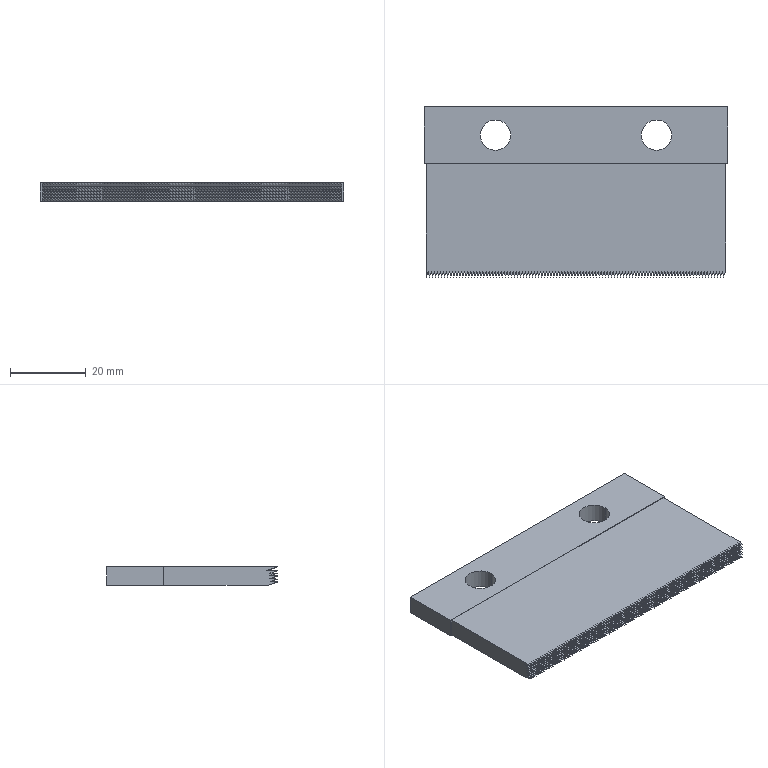Part | SolidWorks | features ICE 3, Extrusion 1, LPattern 1 | 1 solid | 1213 faces | box 80 x 45 x 5 mm | volume 16384 mm3 | plane 1209 | cylinder 4 | commonest cylinder face diameters 8 x4